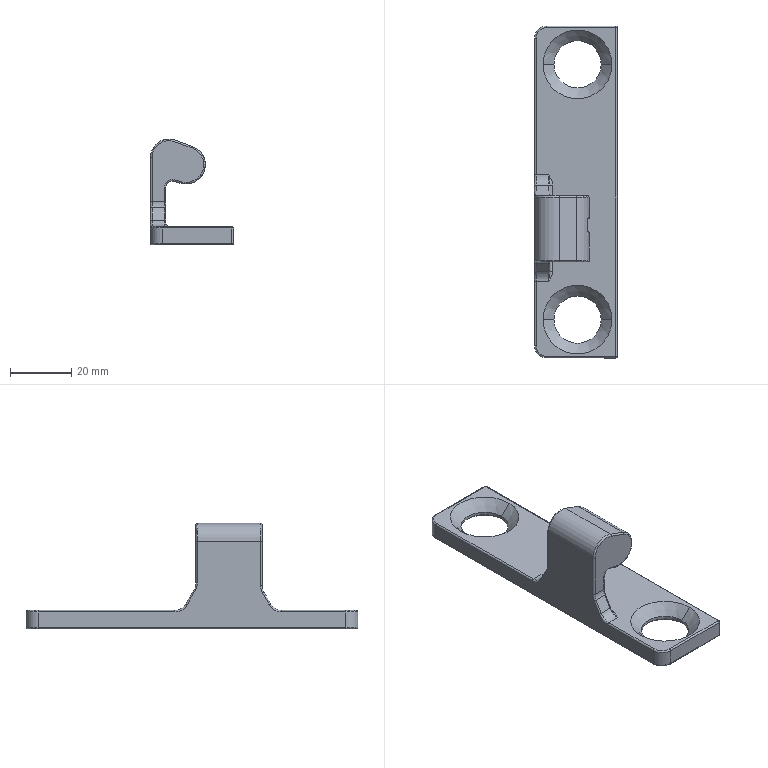Part | NX | features solid 2 | 1 solid | 143 faces | box 27 x 107.982 x 34.413 mm | volume 19876 mm3 | cylinder 51 | plane 39 | torus 26 | spline 19 | sphere 4 | cone 4 | commonest cylinder face diameters 1 x23 0.6 x6 8 x6 15.4 x4 19 x4 6.1 x2